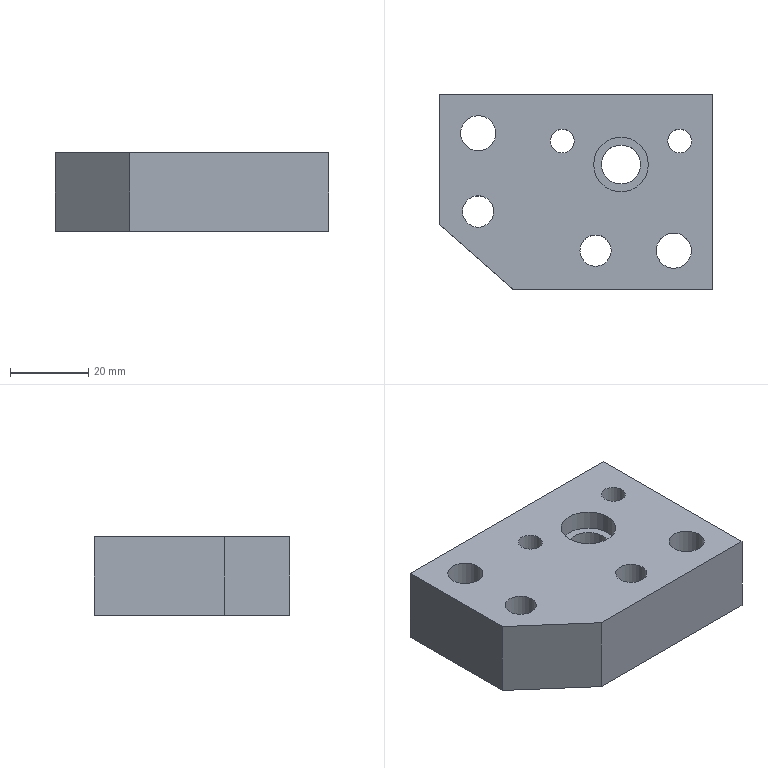Part | STEP file | 426_id2586_x_t | 1 solid | 24 faces | box 70 x 50 x 20 mm | volume 56753 mm3 | cylinder 12 | plane 11 | spline 1 | commonest cylinder face diameters 10 x3 14 x3 6.1 x2 8 x2 9 x2